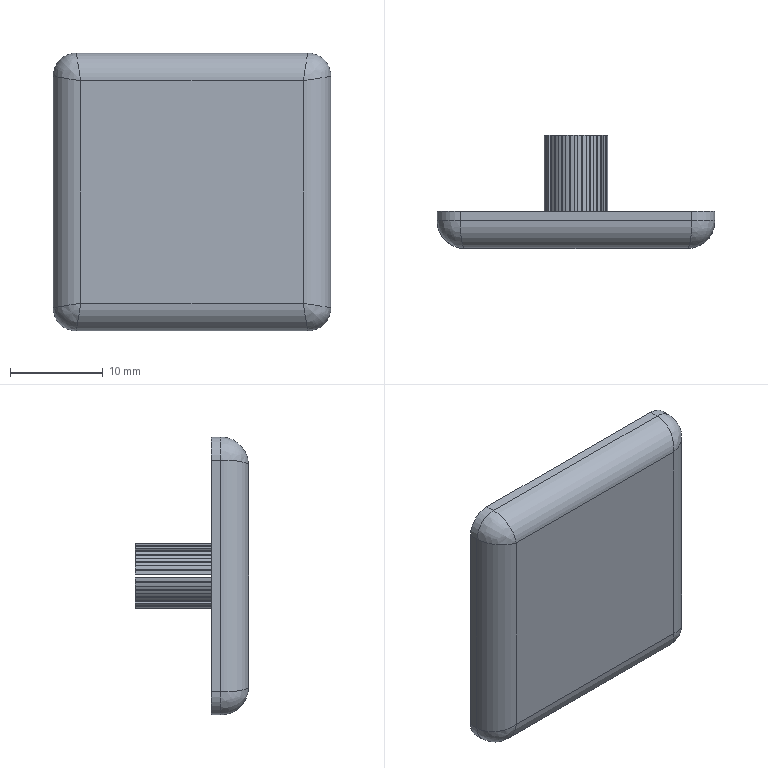Part | STEP file | end cap panel MK-EC-B-3030x4 | 1 solid | 127 faces | box 30 x 12.2 x 30 mm | volume 2778 mm3 | cylinder 62 | plane 61 | spline 4 | commonest cylinder face diameters 6.6 x24 7 x23 5 x8 6 x4 4.9 x3